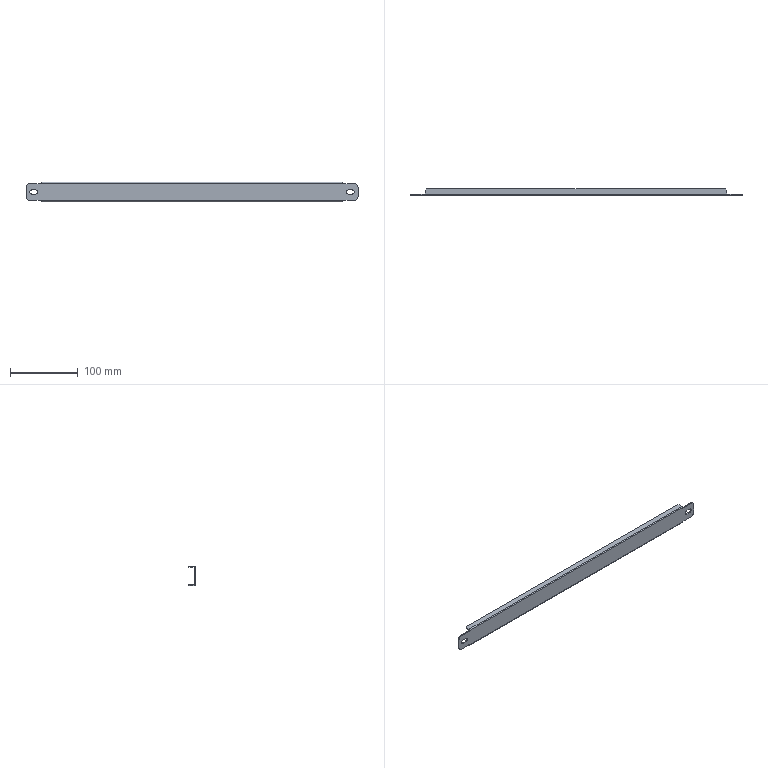Part | SolidWorks | features CornerTrim 2, ICE 2, EdgeFlange 1, FlatPattern 1, SMBaseFlange 1, SheetMetal 1 | 1 solid | 46 faces | box 490 x 9.5 x 29 mm | volume 30933 mm3 | plane 34 | cylinder 12 | commonest cylinder face diameters 6 x4 10 x4 0.2 x2 3.2 x2
STEP:
#1=CARTESIAN_POINT('',(222.5,-1.5,12.));
#2=VERTEX_POINT('',#1);
#3=CARTESIAN_POINT('',(240.,-1.5,12.));
#4=VERTEX_POINT('',#3);
#5=CARTESIAN_POINT('',(-245.,-1.5,12.));
#6=DIRECTION('',(1.,0.,0.));
#7=VECTOR('',#6,1000.);
#8=LINE('',#5,#7);
#9=EDGE_CURVE('',#2,#4,#8,.T.);
#10=ORIENTED_EDGE('',*,*,#9,.T.);
#11=CARTESIAN_POINT('',(240.,0.,12.));
#12=VERTEX_POINT('',#11);
#13=CARTESIAN_POINT('',(240.,-1.5,12.));
#14=DIRECTION('',(0.,1.,0.));
#15=VECTOR('',#14,1000.);
#16=LINE('',#13,#15);
#17=EDGE_CURVE('',#4,#12,#16,.T.);
#18=ORIENTED_EDGE('',*,*,#17,.T.);
#19=CARTESIAN_POINT('',(222.5,0.,12.));
#20=VERTEX_POINT('',#19);
#21=CARTESIAN_POINT('',(-245.,0.,12.));
#22=DIRECTION('',(1.,0.,0.));
#23=VECTOR('',#22,1000.);
#24=LINE('',#21,#23);
#25=EDGE_CURVE('',#20,#12,#24,.T.);
#26=ORIENTED_EDGE('',*,*,#25,.F.);
#27=CARTESIAN_POINT('',(222.5,0.,12.));
#28=DIRECTION('',(0.,-1.,0.));
#29=VECTOR('',#28,1000.);
#30=LINE('',#27,#29);
#31=EDGE_CURVE('',#20,#2,#30,.T.);
#32=ORIENTED_EDGE('',*,*,#31,.T.);
#33=EDGE_LOOP('',(#10,#18,#26,#32));
#34=FACE_OUTER_BOUND('',#33,.T.);
#35=CARTESIAN_POINT('',(-245.,-1.5,12.));
#36=DIRECTION('',(0.,0.,1.));
#37=DIRECTION('',(1.,0.,0.));
#38=AXIS2_PLACEMENT_3D('',#35,#36,#37);
#39=PLANE('',#38);
#40=ADVANCED_FACE('',(#34),#39,.T.);
#41=CARTESIAN_POINT('',(-222.5,-1.5,-12.));
#42=VERTEX_POINT('',#41);
#43=CARTESIAN_POINT('',(-240.,-1.5,-12.));
#44=VERTEX_POINT('',#43);
#45=CARTESIAN_POINT('',(-245.,-1.5,-12.));
#46=DIRECTION('',(-1.,0.,0.));
#47=VECTOR('',#46,1000.);
#48=LINE('',#45,#47);
#49=EDGE_CURVE('',#42,#44,#48,.T.);
#50=ORIENTED_EDGE('',*,*,#49,.T.);
#51=CARTESIAN_POINT('',(-240.,0.,-12.));
#52=VERTEX_POINT('',#51);
#53=CARTESIAN_POINT('',(-240.,-1.5,-12.));
#54=DIRECTION('',(0.,1.,0.));
#55=VECTOR('',#54,1000.);
#56=LINE('',#53,#55);
#57=EDGE_CURVE('',#44,#52,#56,.T.);
#58=ORIENTED_EDGE('',*,*,#57,.T.);
#59=CARTESIAN_POINT('',(-222.5,0.,-12.));
#60=VERTEX_POINT('',#59);
#61=CARTESIAN_POINT('',(-245.,0.,-12.));
#62=DIRECTION('',(-1.,0.,0.));
#63=VECTOR('',#62,1000.);
#64=LINE('',#61,#63);
#65=EDGE_CURVE('',#60,#52,#64,.T.);
#66=ORIENTED_EDGE('',*,*,#65,.F.);
#67=CARTESIAN_POINT('',(-222.5,0.,-12.));
#68=DIRECTION('',(0.,-1.,0.));
#69=VECTOR('',#68,1000.);
#70=LINE('',#67,#69);
#71=EDGE_CURVE('',#60,#42,#70,.T.);
#72=ORIENTED_EDGE('',*,*,#71,.T.);
#73=EDGE_LOOP('',(#50,#58,#66,#72));
#74=FACE_OUTER_BOUND('',#73,.T.);
#75=CARTESIAN_POINT('',(-245.,-1.5,-12.));
#76=DIRECTION('',(0.,0.,-1.));
#77=DIRECTION('',(-1.,0.,0.));
#78=AXIS2_PLACEMENT_3D('',#75,#76,#77);
#79=PLANE('',#78);
#80=ADVANCED_FACE('',(#74),#79,.T.);
#81=CARTESIAN_POINT('',(245.,0.,7.));
#82=VERTEX_POINT('',#81);
#83=CARTESIAN_POINT('',(245.,0.,-7.));
#84=VERTEX_POINT('',#83);
#85=CARTESIAN_POINT('',(245.,0.,-12.));
#86=DIRECTION('',(0.,0.,-1.));
#87=VECTOR('',#86,1000.);
#88=LINE('',#85,#87);
#89=EDGE_CURVE('',#82,#84,#88,.T.);
#90=ORIENTED_EDGE('',*,*,#89,.F.);
#91=CARTESIAN_POINT('',(245.,-1.5,7.));
#92=VERTEX_POINT('',#91);
#93=CARTESIAN_POINT('',(245.,-1.5,7.));
#94=DIRECTION('',(0.,-1.,0.));
#95=VECTOR('',#94,1000.);
#96=LINE('',#93,#95);
#97=EDGE_CURVE('',#82,#92,#96,.T.);
#98=ORIENTED_EDGE('',*,*,#97,.T.);
#99=CARTESIAN_POINT('',(245.,-1.5,-7.));
#100=VERTEX_POINT('',#99);
#101=CARTESIAN_POINT('',(245.,-1.5,-12.));
#102=DIRECTION('',(0.,0.,-1.));
#103=VECTOR('',#102,1000.);
#104=LINE('',#101,#103);
#105=EDGE_CURVE('',#92,#100,#104,.T.);
#106=ORIENTED_EDGE('',*,*,#105,.T.);
#107=CARTESIAN_POINT('',(245.,-1.5,-7.));
#108=DIRECTION('',(0.,1.,0.));
#109=VECTOR('',#108,1000.);
#110=LINE('',#107,#109);
#111=EDGE_CURVE('',#100,#84,#110,.T.);
#112=ORIENTED_EDGE('',*,*,#111,.T.);
#113=EDGE_LOOP('',(#90,#98,#106,#112));
#114=FACE_OUTER_BOUND('',#113,.T.);
#115=CARTESIAN_POINT('',(245.,-1.5,-12.));
#116=DIRECTION('',(1.,0.,0.));
#117=DIRECTION('',(0.,0.,-1.));
#118=AXIS2_PLACEMENT_3D('',#115,#116,#117);
#119=PLANE('',#118);
#120=ADVANCED_FACE('',(#114),#119,.T.);
#121=CARTESIAN_POINT('',(-240.,0.,12.));
#122=VERTEX_POINT('',#121);
#123=CARTESIAN_POINT('',(-222.5,0.,12.));
#124=VERTEX_POINT('',#123);
#125=CARTESIAN_POINT('',(-245.,0.,12.));
#126=DIRECTION('',(1.,0.,0.));
#127=VECTOR('',#126,1000.);
#128=LINE('',#125,#127);
#129=EDGE_CURVE('',#122,#124,#128,.T.);
#130=ORIENTED_EDGE('',*,*,#129,.F.);
#131=CARTESIAN_POINT('',(-240.,-1.5,12.));
#132=VERTEX_POINT('',#131);
#133=CARTESIAN_POINT('',(-240.,-1.5,12.));
#134=DIRECTION('',(0.,-1.,0.));
#135=VECTOR('',#134,1000.);
#136=LINE('',#133,#135);
#137=EDGE_CURVE('',#122,#132,#136,.T.);
#138=ORIENTED_EDGE('',*,*,#137,.T.);
#139=CARTESIAN_POINT('',(-222.5,-1.5,12.));
#140=VERTEX_POINT('',#139);
#141=CARTESIAN_POINT('',(-245.,-1.5,12.));
#142=DIRECTION('',(1.,0.,0.));
#143=VECTOR('',#142,1000.);
#144=LINE('',#141,#143);
#145=EDGE_CURVE('',#132,#140,#144,.T.);
#146=ORIENTED_EDGE('',*,*,#145,.T.);
#147=CARTESIAN_POINT('',(-222.5,0.,12.));
#148=DIRECTION('',(0.,-1.,0.));
#149=VECTOR('',#148,1000.);
#150=LINE('',#147,#149);
#151=EDGE_CURVE('',#124,#140,#150,.T.);
#152=ORIENTED_EDGE('',*,*,#151,.F.);
#153=EDGE_LOOP('',(#130,#138,#146,#152));
#154=FACE_OUTER_BOUND('',#153,.T.);
#155=CARTESIAN_POINT('',(-245.,-1.5,12.));
#156=DIRECTION('',(0.,0.,1.));
#157=DIRECTION('',(1.,0.,0.));
#158=AXIS2_PLACEMENT_3D('',#155,#156,#157);
#159=PLANE('',#158);
#160=ADVANCED_FACE('',(#154),#159,.T.);
#161=CARTESIAN_POINT('',(-245.,-1.5,-7.));
#162=VERTEX_POINT('',#161);
#163=CARTESIAN_POINT('',(-245.,-1.5,7.));
#164=VERTEX_POINT('',#163);
#165=CARTESIAN_POINT('',(-245.,-1.5,-12.));
#166=DIRECTION('',(0.,0.,1.));
#167=VECTOR('',#166,1000.);
#168=LINE('',#165,#167);
#169=EDGE_CURVE('',#162,#164,#168,.T.);
#170=ORIENTED_EDGE('',*,*,#169,.T.);
#171=CARTESIAN_POINT('',(-245.,0.,7.));
#172=VERTEX_POINT('',#171);
#173=CARTESIAN_POINT('',(-245.,-1.5,7.));
#174=DIRECTION('',(0.,1.,0.));
#175=VECTOR('',#174,1000.);
#176=LINE('',#173,#175);
#177=EDGE_CURVE('',#164,#172,#176,.T.);
#178=ORIENTED_EDGE('',*,*,#177,.T.);
#179=CARTESIAN_POINT('',(-245.,0.,-7.));
#180=VERTEX_POINT('',#179);
#181=CARTESIAN_POINT('',(-245.,0.,-12.));
#182=DIRECTION('',(0.,0.,1.));
#183=VECTOR('',#182,1000.);
#184=LINE('',#181,#183);
#185=EDGE_CURVE('',#180,#172,#184,.T.);
#186=ORIENTED_EDGE('',*,*,#185,.F.);
#187=CARTESIAN_POINT('',(-245.,-1.5,-7.));
#188=DIRECTION('',(0.,-1.,0.));
#189=VECTOR('',#188,1000.);
#190=LINE('',#187,#189);
#191=EDGE_CURVE('',#180,#162,#190,.T.);
#192=ORIENTED_EDGE('',*,*,#191,.T.);
#193=EDGE_LOOP('',(#170,#178,#186,#192));
#194=FACE_OUTER_BOUND('',#193,.T.);
#195=CARTESIAN_POINT('',(-245.,-1.5,-12.));
#196=DIRECTION('',(-1.,0.,0.));
#197=DIRECTION('',(0.,0.,1.));
#198=AXIS2_PLACEMENT_3D('',#195,#196,#197);
#199=PLANE('',#198);
#200=ADVANCED_FACE('',(#194),#199,.T.);
#201=CARTESIAN_POINT('',(240.,0.,-12.));
#202=VERTEX_POINT('',#201);
#203=CARTESIAN_POINT('',(222.5,0.,-12.));
#204=VERTEX_POINT('',#203);
#205=CARTESIAN_POINT('',(-245.,0.,-12.));
#206=DIRECTION('',(-1.,0.,0.));
#207=VECTOR('',#206,1000.);
#208=LINE('',#205,#207);
#209=EDGE_CURVE('',#202,#204,#208,.T.);
#210=ORIENTED_EDGE('',*,*,#209,.F.);
#211=CARTESIAN_POINT('',(240.,-1.5,-12.));
#212=VERTEX_POINT('',#211);
#213=CARTESIAN_POINT('',(240.,-1.5,-12.));
#214=DIRECTION('',(0.,-1.,0.));
#215=VECTOR('',#214,1000.);
#216=LINE('',#213,#215);
#217=EDGE_CURVE('',#202,#212,#216,.T.);
#218=ORIENTED_EDGE('',*,*,#217,.T.);
#219=CARTESIAN_POINT('',(222.5,-1.5,-12.));
#220=VERTEX_POINT('',#219);
#221=CARTESIAN_POINT('',(-245.,-1.5,-12.));
#222=DIRECTION('',(-1.,0.,0.));
#223=VECTOR('',#222,1000.);
#224=LINE('',#221,#223);
#225=EDGE_CURVE('',#212,#220,#224,.T.);
#226=ORIENTED_EDGE('',*,*,#225,.T.);
#227=CARTESIAN_POINT('',(222.5,0.,-12.));
#228=DIRECTION('',(0.,-1.,0.));
#229=VECTOR('',#228,1000.);
#230=LINE('',#227,#229);
#231=EDGE_CURVE('',#204,#220,#230,.T.);
#232=ORIENTED_EDGE('',*,*,#231,.F.);
#233=EDGE_LOOP('',(#210,#218,#226,#232));
#234=FACE_OUTER_BOUND('',#233,.T.);
#235=CARTESIAN_POINT('',(-245.,-1.5,-12.));
#236=DIRECTION('',(0.,0.,-1.));
#237=DIRECTION('',(-1.,0.,0.));
#238=AXIS2_PLACEMENT_3D('',#235,#236,#237);
#239=PLANE('',#238);
#240=ADVANCED_FACE('',(#234),#239,.T.);
#241=CARTESIAN_POINT('',(230.5,-1.5,3.));
#242=VERTEX_POINT('',#241);
#243=CARTESIAN_POINT('',(236.5,-1.5,3.));
#244=VERTEX_POINT('',#243);
#245=CARTESIAN_POINT('',(0.,-1.5,3.));
#246=DIRECTION('',(1.,0.,0.));
#247=VECTOR('',#246,1000.);
#248=LINE('',#245,#247);
#249=EDGE_CURVE('',#242,#244,#248,.T.);
#250=ORIENTED_EDGE('',*,*,#249,.T.);
#251=CARTESIAN_POINT('',(236.5,-1.5,-3.));
#252=VERTEX_POINT('',#251);
#253=CARTESIAN_POINT('',(236.5,-1.5,0.));
#254=DIRECTION('',(0.,1.,0.));
#255=DIRECTION('',(0.,0.,1.));
#256=AXIS2_PLACEMENT_3D('',#253,#254,#255);
#257=CIRCLE('',#256,3.);
#258=EDGE_CURVE('',#244,#252,#257,.T.);
#259=ORIENTED_EDGE('',*,*,#258,.T.);
#260=CARTESIAN_POINT('',(230.5,-1.5,-3.));
#261=VERTEX_POINT('',#260);
#262=CARTESIAN_POINT('',(0.,-1.5,-3.));
#263=DIRECTION('',(-1.,0.,0.));
#264=VECTOR('',#263,1000.);
#265=LINE('',#262,#264);
#266=EDGE_CURVE('',#252,#261,#265,.T.);
#267=ORIENTED_EDGE('',*,*,#266,.T.);
#268=CARTESIAN_POINT('',(230.5,-1.5,0.));
#269=DIRECTION('',(0.,1.,0.));
#270=DIRECTION('',(0.,0.,1.));
#271=AXIS2_PLACEMENT_3D('',#268,#269,#270);
#272=CIRCLE('',#271,3.);
#273=EDGE_CURVE('',#261,#242,#272,.T.);
#274=ORIENTED_EDGE('',*,*,#273,.T.);
#275=EDGE_LOOP('',(#250,#259,#267,#274));
#276=FACE_BOUND('',#275,.T.);
#277=CARTESIAN_POINT('',(-236.5,-1.5,3.));
#278=VERTEX_POINT('',#277);
#279=CARTESIAN_POINT('',(-230.5,-1.5,3.));
#280=VERTEX_POINT('',#279);
#281=CARTESIAN_POINT('',(0.,-1.5,3.));
#282=DIRECTION('',(1.,0.,0.));
#283=VECTOR('',#282,1000.);
#284=LINE('',#281,#283);
#285=EDGE_CURVE('',#278,#280,#284,.T.);
#286=ORIENTED_EDGE('',*,*,#285,.T.);
#287=CARTESIAN_POINT('',(-230.5,-1.5,-3.));
#288=VERTEX_POINT('',#287);
#289=CARTESIAN_POINT('',(-230.5,-1.5,0.));
#290=DIRECTION('',(0.,1.,0.));
#291=DIRECTION('',(0.,0.,1.));
#292=AXIS2_PLACEMENT_3D('',#289,#290,#291);
#293=CIRCLE('',#292,3.);
#294=EDGE_CURVE('',#280,#288,#293,.T.);
#295=ORIENTED_EDGE('',*,*,#294,.T.);
#296=CARTESIAN_POINT('',(-236.5,-1.5,-3.));
#297=VERTEX_POINT('',#296);
#298=CARTESIAN_POINT('',(0.,-1.5,-3.));
#299=DIRECTION('',(-1.,0.,0.));
#300=VECTOR('',#299,1000.);
#301=LINE('',#298,#300);
#302=EDGE_CURVE('',#288,#297,#301,.T.);
#303=ORIENTED_EDGE('',*,*,#302,.T.);
#304=CARTESIAN_POINT('',(-236.5,-1.5,0.));
#305=DIRECTION('',(0.,1.,0.));
#306=DIRECTION('',(0.,0.,1.));
#307=AXIS2_PLACEMENT_3D('',#304,#305,#306);
#308=CIRCLE('',#307,3.);
#309=EDGE_CURVE('',#297,#278,#308,.T.);
#310=ORIENTED_EDGE('',*,*,#309,.T.);
#311=EDGE_LOOP('',(#286,#295,#303,#310));
#312=FACE_BOUND('',#311,.T.);
#313=ORIENTED_EDGE('',*,*,#105,.F.);
#314=CARTESIAN_POINT('',(240.,-1.5,7.));
#315=DIRECTION('',(0.,-1.,0.));
#316=DIRECTION('',(0.,0.,1.));
#317=AXIS2_PLACEMENT_3D('',#314,#315,#316);
#318=CIRCLE('',#317,5.);
#319=EDGE_CURVE('',#92,#4,#318,.T.);
#320=ORIENTED_EDGE('',*,*,#319,.T.);
#321=ORIENTED_EDGE('',*,*,#9,.F.);
#322=CARTESIAN_POINT('',(222.5,-1.5,12.9));
#323=VERTEX_POINT('',#322);
#324=CARTESIAN_POINT('',(222.5,-1.5,12.9));
#325=DIRECTION('',(0.,0.,-1.));
#326=VECTOR('',#325,1000.);
#327=LINE('',#324,#326);
#328=EDGE_CURVE('',#323,#2,#327,.T.);
#329=ORIENTED_EDGE('',*,*,#328,.F.);
#330=CARTESIAN_POINT('',(-222.5,-1.5,12.9));
#331=VERTEX_POINT('',#330);
#332=CARTESIAN_POINT('',(222.5,-1.5,12.9));
#333=DIRECTION('',(-1.,0.,0.));
#334=VECTOR('',#333,1000.);
#335=LINE('',#332,#334);
#336=EDGE_CURVE('',#323,#331,#335,.T.);
#337=ORIENTED_EDGE('',*,*,#336,.T.);
#338=CARTESIAN_POINT('',(-222.5,-1.5,12.9));
#339=DIRECTION('',(0.,0.,-1.));
#340=VECTOR('',#339,1000.);
#341=LINE('',#338,#340);
#342=EDGE_CURVE('',#331,#140,#341,.T.);
#343=ORIENTED_EDGE('',*,*,#342,.T.);
#344=ORIENTED_EDGE('',*,*,#145,.F.);
#345=CARTESIAN_POINT('',(-240.,-1.5,7.));
#346=DIRECTION('',(0.,-1.,0.));
#347=DIRECTION('',(0.,0.,1.));
#348=AXIS2_PLACEMENT_3D('',#345,#346,#347);
#349=CIRCLE('',#348,5.);
#350=EDGE_CURVE('',#132,#164,#349,.T.);
#351=ORIENTED_EDGE('',*,*,#350,.T.);
#352=ORIENTED_EDGE('',*,*,#169,.F.);
#353=CARTESIAN_POINT('',(-240.,-1.5,-7.));
#354=DIRECTION('',(0.,-1.,0.));
#355=DIRECTION('',(0.,0.,1.));
#356=AXIS2_PLACEMENT_3D('',#353,#354,#355);
#357=CIRCLE('',#356,5.);
#358=EDGE_CURVE('',#162,#44,#357,.T.);
#359=ORIENTED_EDGE('',*,*,#358,.T.);
#360=ORIENTED_EDGE('',*,*,#49,.F.);
#361=CARTESIAN_POINT('',(-222.5,-1.5,-12.9));
#362=VERTEX_POINT('',#361);
#363=CARTESIAN_POINT('',(-222.5,-1.5,-12.9));
#364=DIRECTION('',(0.,0.,1.));
#365=VECTOR('',#364,1000.);
#366=LINE('',#363,#365);
#367=EDGE_CURVE('',#362,#42,#366,.T.);
#368=ORIENTED_EDGE('',*,*,#367,.F.);
#369=CARTESIAN_POINT('',(222.5,-1.5,-12.9));
#370=VERTEX_POINT('',#369);
#371=CARTESIAN_POINT('',(-222.5,-1.5,-12.9));
#372=DIRECTION('',(1.,0.,0.));
#373=VECTOR('',#372,1000.);
#374=LINE('',#371,#373);
#375=EDGE_CURVE('',#362,#370,#374,.T.);
#376=ORIENTED_EDGE('',*,*,#375,.T.);
#377=CARTESIAN_POINT('',(222.5,-1.5,-12.9));
#378=DIRECTION('',(0.,0.,1.));
#379=VECTOR('',#378,1000.);
#380=LINE('',#377,#379);
#381=EDGE_CURVE('',#370,#220,#380,.T.);
#382=ORIENTED_EDGE('',*,*,#381,.T.);
#383=ORIENTED_EDGE('',*,*,#225,.F.);
#384=CARTESIAN_POINT('',(240.,-1.5,-7.));
#385=DIRECTION('',(0.,-1.,0.));
#386=DIRECTION('',(0.,0.,1.));
#387=AXIS2_PLACEMENT_3D('',#384,#385,#386);
#388=CIRCLE('',#387,5.);
#389=EDGE_CURVE('',#212,#100,#388,.T.);
#390=ORIENTED_EDGE('',*,*,#389,.T.);
#391=EDGE_LOOP('',(#313,#320,#321,#329,#337,#343,#344,#351,#352,#359,#360,#368,#376,#382,#383,#390));
#392=FACE_OUTER_BOUND('',#391,.T.);
#393=CARTESIAN_POINT('',(0.,-1.5,0.));
#394=DIRECTION('',(0.,1.,0.));
#395=DIRECTION('',(0.,0.,1.));
#396=AXIS2_PLACEMENT_3D('',#393,#394,#395);
#397=PLANE('',#396);
#398=ADVANCED_FACE('',(#276,#312,#392),#397,.F.);
#399=CARTESIAN_POINT('',(236.5,0.,3.));
#400=VERTEX_POINT('',#399);
#401=CARTESIAN_POINT('',(236.5,0.,-3.));
#402=VERTEX_POINT('',#401);
#403=CARTESIAN_POINT('',(236.5,0.,0.));
#404=DIRECTION('',(0.,1.,0.));
#405=DIRECTION('',(0.,0.,1.));
#406=AXIS2_PLACEMENT_3D('',#403,#404,#405);
#407=CIRCLE('',#406,3.);
#408=EDGE_CURVE('',#400,#402,#407,.T.);
#409=ORIENTED_EDGE('',*,*,#408,.F.);
#410=CARTESIAN_POINT('',(230.5,0.,3.));
#411=VERTEX_POINT('',#410);
#412=CARTESIAN_POINT('',(236.5,0.,3.));
#413=DIRECTION('',(1.,0.,0.));
#414=VECTOR('',#413,1000.);
#415=LINE('',#412,#414);
#416=EDGE_CURVE('',#411,#400,#415,.T.);
#417=ORIENTED_EDGE('',*,*,#416,.F.);
#418=CARTESIAN_POINT('',(230.5,0.,-3.));
#419=VERTEX_POINT('',#418);
#420=CARTESIAN_POINT('',(230.5,0.,0.));
#421=DIRECTION('',(0.,1.,0.));
#422=DIRECTION('',(0.,0.,1.));
#423=AXIS2_PLACEMENT_3D('',#420,#421,#422);
#424=CIRCLE('',#423,3.);
#425=EDGE_CURVE('',#419,#411,#424,.T.);
#426=ORIENTED_EDGE('',*,*,#425,.F.);
#427=CARTESIAN_POINT('',(236.5,0.,-3.));
#428=DIRECTION('',(-1.,0.,0.));
#429=VECTOR('',#428,1000.);
#430=LINE('',#427,#429);
#431=EDGE_CURVE('',#402,#419,#430,.T.);
#432=ORIENTED_EDGE('',*,*,#431,.F.);
#433=EDGE_LOOP('',(#409,#417,#426,#432));
#434=FACE_BOUND('',#433,.T.);
#435=CARTESIAN_POINT('',(-230.5,0.,3.));
#436=VERTEX_POINT('',#435);
#437=CARTESIAN_POINT('',(-230.5,0.,-3.));
#438=VERTEX_POINT('',#437);
#439=CARTESIAN_POINT('',(-230.5,0.,0.));
#440=DIRECTION('',(0.,1.,0.));
#441=DIRECTION('',(0.,0.,1.));
#442=AXIS2_PLACEMENT_3D('',#439,#440,#441);
#443=CIRCLE('',#442,3.);
#444=EDGE_CURVE('',#436,#438,#443,.T.);
#445=ORIENTED_EDGE('',*,*,#444,.F.);
#446=CARTESIAN_POINT('',(-236.5,0.,3.));
#447=VERTEX_POINT('',#446);
#448=CARTESIAN_POINT('',(-230.5,0.,3.));
#449=DIRECTION('',(1.,0.,0.));
#450=VECTOR('',#449,1000.);
#451=LINE('',#448,#450);
#452=EDGE_CURVE('',#447,#436,#451,.T.);
#453=ORIENTED_EDGE('',*,*,#452,.F.);
#454=CARTESIAN_POINT('',(-236.5,0.,-3.));
#455=VERTEX_POINT('',#454);
#456=CARTESIAN_POINT('',(-236.5,0.,0.));
#457=DIRECTION('',(0.,1.,0.));
#458=DIRECTION('',(0.,0.,1.));
#459=AXIS2_PLACEMENT_3D('',#456,#457,#458);
#460=CIRCLE('',#459,3.);
#461=EDGE_CURVE('',#455,#447,#460,.T.);
#462=ORIENTED_EDGE('',*,*,#461,.F.);
#463=CARTESIAN_POINT('',(-230.5,0.,-3.));
#464=DIRECTION('',(-1.,0.,0.));
#465=VECTOR('',#464,1000.);
#466=LINE('',#463,#465);
#467=EDGE_CURVE('',#438,#455,#466,.T.);
#468=ORIENTED_EDGE('',*,*,#467,.F.);
#469=EDGE_LOOP('',(#445,#453,#462,#468));
#470=FACE_BOUND('',#469,.T.);
#471=ORIENTED_EDGE('',*,*,#25,.T.);
#472=CARTESIAN_POINT('',(240.,0.,7.));
#473=DIRECTION('',(0.,1.,0.));
#474=DIRECTION('',(0.,0.,1.));
#475=AXIS2_PLACEMENT_3D('',#472,#473,#474);
#476=CIRCLE('',#475,5.);
#477=EDGE_CURVE('',#12,#82,#476,.T.);
#478=ORIENTED_EDGE('',*,*,#477,.T.);
#479=ORIENTED_EDGE('',*,*,#89,.T.);
#480=CARTESIAN_POINT('',(240.,0.,-7.));
#481=DIRECTION('',(0.,1.,0.));
#482=DIRECTION('',(0.,0.,1.));
#483=AXIS2_PLACEMENT_3D('',#480,#481,#482);
#484=CIRCLE('',#483,5.);
#485=EDGE_CURVE('',#84,#202,#484,.T.);
#486=ORIENTED_EDGE('',*,*,#485,.T.);
#487=ORIENTED_EDGE('',*,*,#209,.T.);
#488=CARTESIAN_POINT('',(222.5,0.,-12.9));
#489=VERTEX_POINT('',#488);
#490=CARTESIAN_POINT('',(222.5,0.,-12.9));
#491=DIRECTION('',(0.,0.,1.));
#492=VECTOR('',#491,1000.);
#493=LINE('',#490,#492);
#494=EDGE_CURVE('',#489,#204,#493,.T.);
#495=ORIENTED_EDGE('',*,*,#494,.F.);
#496=CARTESIAN_POINT('',(-222.5,0.,-12.9));
#497=VERTEX_POINT('',#496);
#498=CARTESIAN_POINT('',(-222.5,0.,-12.9));
#499=DIRECTION('',(1.,0.,0.));
#500=VECTOR('',#499,1000.);
#501=LINE('',#498,#500);
#502=EDGE_CURVE('',#497,#489,#501,.T.);
#503=ORIENTED_EDGE('',*,*,#502,.F.);
#504=CARTESIAN_POINT('',(-222.5,0.,-12.9));
#505=DIRECTION('',(0.,0.,1.));
#506=VECTOR('',#505,1000.);
#507=LINE('',#504,#506);
#508=EDGE_CURVE('',#497,#60,#507,.T.);
#509=ORIENTED_EDGE('',*,*,#508,.T.);
#510=ORIENTED_EDGE('',*,*,#65,.T.);
#511=CARTESIAN_POINT('',(-240.,0.,-7.));
#512=DIRECTION('',(0.,1.,0.));
#513=DIRECTION('',(0.,0.,1.));
#514=AXIS2_PLACEMENT_3D('',#511,#512,#513);
#515=CIRCLE('',#514,5.);
#516=EDGE_CURVE('',#52,#180,#515,.T.);
#517=ORIENTED_EDGE('',*,*,#516,.T.);
#518=ORIENTED_EDGE('',*,*,#185,.T.);
#519=CARTESIAN_POINT('',(-240.,0.,7.));
#520=DIRECTION('',(0.,1.,0.));
#521=DIRECTION('',(0.,0.,1.));
#522=AXIS2_PLACEMENT_3D('',#519,#520,#521);
#523=CIRCLE('',#522,5.);
#524=EDGE_CURVE('',#172,#122,#523,.T.);
#525=ORIENTED_EDGE('',*,*,#524,.T.);
#526=ORIENTED_EDGE('',*,*,#129,.T.);
#527=CARTESIAN_POINT('',(-222.5,0.,12.9));
#528=VERTEX_POINT('',#527);
#529=CARTESIAN_POINT('',(-222.5,0.,12.9));
#530=DIRECTION('',(0.,0.,-1.));
#531=VECTOR('',#530,1000.);
#532=LINE('',#529,#531);
#533=EDGE_CURVE('',#528,#124,#532,.T.);
#534=ORIENTED_EDGE('',*,*,#533,.F.);
#535=CARTESIAN_POINT('',(222.5,0.,12.9));
#536=VERTEX_POINT('',#535);
#537=CARTESIAN_POINT('',(222.5,0.,12.9));
#538=DIRECTION('',(-1.,0.,0.));
#539=VECTOR('',#538,1000.);
#540=LINE('',#537,#539);
#541=EDGE_CURVE('',#536,#528,#540,.T.);
#542=ORIENTED_EDGE('',*,*,#541,.F.);
#543=CARTESIAN_POINT('',(222.5,0.,12.9));
#544=DIRECTION('',(0.,0.,-1.));
#545=VECTOR('',#544,1000.);
#546=LINE('',#543,#545);
#547=EDGE_CURVE('',#536,#20,#546,.T.);
#548=ORIENTED_EDGE('',*,*,#547,.T.);
#549=EDGE_LOOP('',(#471,#478,#479,#486,#487,#495,#503,#509,#510,#517,#518,#525,#526,#534,#542,#548));
#550=FACE_OUTER_BOUND('',#549,.T.);
#551=CARTESIAN_POINT('',(0.,0.,0.));
#552=DIRECTION('',(0.,1.,0.));
#553=DIRECTION('',(0.,0.,1.));
#554=AXIS2_PLACEMENT_3D('',#551,#552,#553);
#555=PLANE('',#554);
#556=ADVANCED_FACE('',(#434,#470,#550),#555,.T.);
#557=ORIENTED_EDGE('',*,*,#508,.F.);
#558=CARTESIAN_POINT('',(-222.5,0.,-12.9));
#559=DIRECTION('',(0.,-1.,0.));
#560=VECTOR('',#559,1000.);
#561=LINE('',#558,#560);
#562=EDGE_CURVE('',#497,#362,#561,.T.);
#563=ORIENTED_EDGE('',*,*,#562,.T.);
#564=ORIENTED_EDGE('',*,*,#367,.T.);
#565=ORIENTED_EDGE('',*,*,#71,.F.);
#566=EDGE_LOOP('',(#557,#563,#564,#565));
#567=FACE_OUTER_BOUND('',#566,.T.);
#568=CARTESIAN_POINT('',(-222.5,0.,-12.9));
#569=DIRECTION('',(-1.,0.,0.));
#570=DIRECTION('',(0.,-1.,0.));
#571=AXIS2_PLACEMENT_3D('',#568,#569,#570);
#572=PLANE('',#571);
#573=ADVANCED_FACE('',(#567),#572,.T.);
#574=ORIENTED_EDGE('',*,*,#381,.F.);
#575=CARTESIAN_POINT('',(222.5,0.,-12.9));
#576=DIRECTION('',(0.,-1.,0.));
#577=VECTOR('',#576,1000.);
#578=LINE('',#575,#577);
#579=EDGE_CURVE('',#489,#370,#578,.T.);
#580=ORIENTED_EDGE('',*,*,#579,.F.);
#581=ORIENTED_EDGE('',*,*,#494,.T.);
#582=ORIENTED_EDGE('',*,*,#231,.T.);
#583=EDGE_LOOP('',(#574,#580,#581,#582));
#584=FACE_OUTER_BOUND('',#583,.T.);
#585=CARTESIAN_POINT('',(222.5,0.,-12.9));
#586=DIRECTION('',(-1.,0.,0.));
#587=DIRECTION('',(0.,-1.,0.));
#588=AXIS2_PLACEMENT_3D('',#585,#586,#587);
#589=PLANE('',#588);
#590=ADVANCED_FACE('',(#584),#589,.F.);
#591=ORIENTED_EDGE('',*,*,#547,.F.);
#592=CARTESIAN_POINT('',(222.5,0.,12.9));
#593=DIRECTION('',(0.,-1.,0.));
#594=VECTOR('',#593,1000.);
#595=LINE('',#592,#594);
#596=EDGE_CURVE('',#536,#323,#595,.T.);
#597=ORIENTED_EDGE('',*,*,#596,.T.);
#598=ORIENTED_EDGE('',*,*,#328,.T.);
#599=ORIENTED_EDGE('',*,*,#31,.F.);
#600=EDGE_LOOP('',(#591,#597,#598,#599));
#601=FACE_OUTER_BOUND('',#600,.T.);
#602=CARTESIAN_POINT('',(222.5,0.,12.9));
#603=DIRECTION('',(1.,0.,0.));
#604=DIRECTION('',(0.,-1.,0.));
#605=AXIS2_PLACEMENT_3D('',#602,#603,#604);
#606=PLANE('',#605);
#607=ADVANCED_FACE('',(#601),#606,.T.);
#608=ORIENTED_EDGE('',*,*,#342,.F.);
#609=CARTESIAN_POINT('',(-222.5,0.,12.9));
#610=DIRECTION('',(0.,-1.,0.));
#611=VECTOR('',#610,1000.);
#612=LINE('',#609,#611);
#613=EDGE_CURVE('',#528,#331,#612,.T.);
#614=ORIENTED_EDGE('',*,*,#613,.F.);
#615=ORIENTED_EDGE('',*,*,#533,.T.);
#616=ORIENTED_EDGE('',*,*,#151,.T.);
#617=EDGE_LOOP('',(#608,#614,#615,#616));
#618=FACE_OUTER_BOUND('',#617,.T.);
#619=CARTESIAN_POINT('',(-222.5,0.,12.9));
#620=DIRECTION('',(1.,0.,0.));
#621=DIRECTION('',(0.,-1.,0.));
#622=AXIS2_PLACEMENT_3D('',#619,#620,#621);
#623=PLANE('',#622);
#624=ADVANCED_FACE('',(#618),#623,.F.);
#625=CARTESIAN_POINT('',(222.5,0.1,-13.));
#626=VERTEX_POINT('',#625);
#627=CARTESIAN_POINT('',(222.5,0.1,-14.5));
#628=VERTEX_POINT('',#627);
#629=CARTESIAN_POINT('',(222.5,0.1,-14.5));
#630=DIRECTION('',(0.,0.,-1.));
#631=VECTOR('',#630,1000.);
#632=LINE('',#629,#631);
#633=EDGE_CURVE('',#626,#628,#632,.T.);
#634=ORIENTED_EDGE('',*,*,#633,.F.);
#635=CARTESIAN_POINT('',(222.5,0.1,-12.9));
#636=DIRECTION('',(1.,0.,0.));
#637=DIRECTION('',(0.,-1.,0.));
#638=AXIS2_PLACEMENT_3D('',#635,#636,#637);
#639=CIRCLE('',#638,0.1);
#640=EDGE_CURVE('',#489,#626,#639,.T.);
#641=ORIENTED_EDGE('',*,*,#640,.F.);
#642=ORIENTED_EDGE('',*,*,#579,.T.);
#643=CARTESIAN_POINT('',(222.5,0.1,-12.9));
#644=DIRECTION('',(1.,0.,0.));
#645=DIRECTION('',(0.,-1.,0.));
#646=AXIS2_PLACEMENT_3D('',#643,#644,#645);
#647=CIRCLE('',#646,1.6);
#648=EDGE_CURVE('',#370,#628,#647,.T.);
#649=ORIENTED_EDGE('',*,*,#648,.T.);
#650=EDGE_LOOP('',(#634,#641,#642,#649));
#651=FACE_OUTER_BOUND('',#650,.T.);
#652=CARTESIAN_POINT('',(222.5,0.1,-12.9));
#653=DIRECTION('',(1.,0.,0.));
#654=DIRECTION('',(0.,1.,0.));
#655=AXIS2_PLACEMENT_3D('',#652,#653,#654);
#656=PLANE('',#655);
#657=ADVANCED_FACE('',(#651),#656,.T.);
#658=CARTESIAN_POINT('',(-222.5,0.1,-13.));
#659=VERTEX_POINT('',#658);
#660=CARTESIAN_POINT('',(-222.5,0.1,-12.9));
#661=DIRECTION('',(-1.,0.,0.));
#662=DIRECTION('',(0.,-1.,0.));
#663=AXIS2_PLACEMENT_3D('',#660,#661,#662);
#664=CIRCLE('',#663,0.1);
#665=EDGE_CURVE('',#659,#497,#664,.T.);
#666=ORIENTED_EDGE('',*,*,#665,.F.);
#667=CARTESIAN_POINT('',(-222.5,0.1,-14.5));
#668=VERTEX_POINT('',#667);
#669=CARTESIAN_POINT('',(-222.5,0.1,-13.));
#670=DIRECTION('',(0.,0.,-1.));
#671=VECTOR('',#670,1000.);
#672=LINE('',#669,#671);
#673=EDGE_CURVE('',#659,#668,#672,.T.);
#674=ORIENTED_EDGE('',*,*,#673,.T.);
#675=CARTESIAN_POINT('',(-222.5,0.1,-12.9));
#676=DIRECTION('',(-1.,0.,0.));
#677=DIRECTION('',(0.,-1.,0.));
#678=AXIS2_PLACEMENT_3D('',#675,#676,#677);
#679=CIRCLE('',#678,1.6);
#680=EDGE_CURVE('',#668,#362,#679,.T.);
#681=ORIENTED_EDGE('',*,*,#680,.T.);
#682=ORIENTED_EDGE('',*,*,#562,.F.);
#683=EDGE_LOOP('',(#666,#674,#681,#682));
#684=FACE_OUTER_BOUND('',#683,.T.);
#685=CARTESIAN_POINT('',(-222.5,0.1,-12.9));
#686=DIRECTION('',(1.,0.,0.));
#687=DIRECTION('',(0.,1.,0.));
#688=AXIS2_PLACEMENT_3D('',#685,#686,#687);
#689=PLANE('',#688);
#690=ADVANCED_FACE('',(#684),#689,.F.);
#691=ORIENTED_EDGE('',*,*,#375,.F.);
#692=ORIENTED_EDGE('',*,*,#680,.F.);
#693=CARTESIAN_POINT('',(222.5,0.1,-14.5));
#694=DIRECTION('',(1.,0.,0.));
#695=VECTOR('',#694,1000.);
#696=LINE('',#693,#695);
#697=EDGE_CURVE('',#668,#628,#696,.T.);
#698=ORIENTED_EDGE('',*,*,#697,.T.);
#699=ORIENTED_EDGE('',*,*,#648,.F.);
#700=EDGE_LOOP('',(#691,#692,#698,#699));
#701=FACE_OUTER_BOUND('',#700,.T.);
#702=CARTESIAN_POINT('',(-222.5,0.1,-12.9));
#703=DIRECTION('',(-1.,0.,0.));
#704=DIRECTION('',(0.,0.,-1.));
#705=AXIS2_PLACEMENT_3D('',#702,#703,#704);
#706=CYLINDRICAL_SURFACE('',#705,1.6);
#707=ADVANCED_FACE('',(#701),#706,.T.);
#708=ORIENTED_EDGE('',*,*,#502,.T.);
#709=ORIENTED_EDGE('',*,*,#640,.T.);
#710=CARTESIAN_POINT('',(222.5,0.1,-13.));
#711=DIRECTION('',(-1.,0.,0.));
#712=VECTOR('',#711,1000.);
#713=LINE('',#710,#712);
#714=EDGE_CURVE('',#626,#659,#713,.T.);
#715=ORIENTED_EDGE('',*,*,#714,.T.);
#716=ORIENTED_EDGE('',*,*,#665,.T.);
#717=EDGE_LOOP('',(#708,#709,#715,#716));
#718=FACE_OUTER_BOUND('',#717,.T.);
#719=CARTESIAN_POINT('',(-222.5,0.1,-12.9));
#720=DIRECTION('',(-1.,0.,0.));
#721=DIRECTION('',(0.,0.,-1.));
#722=AXIS2_PLACEMENT_3D('',#719,#720,#721);
#723=CYLINDRICAL_SURFACE('',#722,0.1);
#724=ADVANCED_FACE('',(#718),#723,.F.);
#725=CARTESIAN_POINT('',(222.5,6.,-14.5));
#726=VERTEX_POINT('',#725);
#727=CARTESIAN_POINT('',(222.5,0.,-14.5));
#728=DIRECTION('',(0.,-1.,0.));
#729=VECTOR('',#728,1000.);
#730=LINE('',#727,#729);
#731=EDGE_CURVE('',#726,#628,#730,.T.);
#732=ORIENTED_EDGE('',*,*,#731,.F.);
#733=CARTESIAN_POINT('',(222.5,6.,-13.));
#734=VERTEX_POINT('',#733);
#735=CARTESIAN_POINT('',(222.5,6.,-14.5));
#736=DIRECTION('',(0.,0.,1.));
#737=VECTOR('',#736,1000.);
#738=LINE('',#735,#737);
#739=EDGE_CURVE('',#726,#734,#738,.T.);
#740=ORIENTED_EDGE('',*,*,#739,.T.);
#741=CARTESIAN_POINT('',(222.5,0.,-13.));
#742=DIRECTION('',(0.,-1.,0.));
#743=VECTOR('',#742,1000.);
#744=LINE('',#741,#743);
#745=EDGE_CURVE('',#734,#626,#744,.T.);
#746=ORIENTED_EDGE('',*,*,#745,.T.);
#747=ORIENTED_EDGE('',*,*,#633,.T.);
#748=EDGE_LOOP('',(#732,#740,#746,#747));
#749=FACE_OUTER_BOUND('',#748,.T.);
#750=CARTESIAN_POINT('',(222.5,0.,-14.5));
#751=DIRECTION('',(-1.,0.,0.));
#752=DIRECTION('',(0.,0.,1.));
#753=AXIS2_PLACEMENT_3D('',#750,#751,#752);
#754=PLANE('',#753);
#755=ADVANCED_FACE('',(#749),#754,.F.);
#756=CARTESIAN_POINT('',(-222.5,6.,-13.));
#757=VERTEX_POINT('',#756);
#758=CARTESIAN_POINT('',(-222.5,8.,-13.));
#759=DIRECTION('',(0.,1.,0.));
#760=VECTOR('',#759,1000.);
#761=LINE('',#758,#760);
#762=EDGE_CURVE('',#659,#757,#761,.T.);
#763=ORIENTED_EDGE('',*,*,#762,.T.);
#764=CARTESIAN_POINT('',(-222.5,6.,-14.5));
#765=VERTEX_POINT('',#764);
#766=CARTESIAN_POINT('',(-222.5,6.,-14.5));
#767=DIRECTION('',(0.,0.,-1.));
#768=VECTOR('',#767,1000.);
#769=LINE('',#766,#768);
#770=EDGE_CURVE('',#757,#765,#769,.T.);
#771=ORIENTED_EDGE('',*,*,#770,.T.);
#772=CARTESIAN_POINT('',(-222.5,0.,-14.5));
#773=DIRECTION('',(0.,1.,0.));
#774=VECTOR('',#773,1000.);
#775=LINE('',#772,#774);
#776=EDGE_CURVE('',#668,#765,#775,.T.);
#777=ORIENTED_EDGE('',*,*,#776,.F.);
#778=ORIENTED_EDGE('',*,*,#673,.F.);
#779=EDGE_LOOP('',(#763,#771,#777,#778));
#780=FACE_OUTER_BOUND('',#779,.T.);
#781=CARTESIAN_POINT('',(-222.5,8.,-14.5));
#782=DIRECTION('',(1.,0.,0.));
#783=DIRECTION('',(0.,0.,-1.));
#784=AXIS2_PLACEMENT_3D('',#781,#782,#783);
#785=PLANE('',#784);
#786=ADVANCED_FACE('',(#780),#785,.F.);
#787=CARTESIAN_POINT('',(-220.5,8.,-14.5));
#788=VERTEX_POINT('',#787);
#789=CARTESIAN_POINT('',(220.5,8.,-14.5));
#790=VERTEX_POINT('',#789);
#791=CARTESIAN_POINT('',(0.,8.,-14.5));
#792=DIRECTION('',(1.,0.,0.));
#793=VECTOR('',#792,1000.);
#794=LINE('',#791,#793);
#795=EDGE_CURVE('',#788,#790,#794,.T.);
#796=ORIENTED_EDGE('',*,*,#795,.T.);
#797=CARTESIAN_POINT('',(222.5,6.,-14.5));
#798=DIRECTION('',(0.7071,-0.7071,0.));
#799=VECTOR('',#798,1000.);
#800=LINE('',#797,#799);
#801=EDGE_CURVE('',#790,#726,#800,.T.);
#802=ORIENTED_EDGE('',*,*,#801,.T.);
#803=ORIENTED_EDGE('',*,*,#731,.T.);
#804=ORIENTED_EDGE('',*,*,#697,.F.);
#805=ORIENTED_EDGE('',*,*,#776,.T.);
#806=CARTESIAN_POINT('',(-220.5,8.,-14.5));
#807=DIRECTION('',(0.7071,0.7071,0.));
#808=VECTOR('',#807,1000.);
#809=LINE('',#806,#808);
#810=EDGE_CURVE('',#765,#788,#809,.T.);
#811=ORIENTED_EDGE('',*,*,#810,.T.);
#812=EDGE_LOOP('',(#796,#802,#803,#804,#805,#811));
#813=FACE_OUTER_BOUND('',#812,.T.);
#814=CARTESIAN_POINT('',(0.,0.,-14.5));
#815=DIRECTION('',(0.,0.,1.));
#816=DIRECTION('',(0.,-1.,0.));
#817=AXIS2_PLACEMENT_3D('',#814,#815,#816);
#818=PLANE('',#817);
#819=ADVANCED_FACE('',(#813),#818,.F.);
#820=ORIENTED_EDGE('',*,*,#745,.F.);
#821=CARTESIAN_POINT('',(220.5,8.,-13.));
#822=VERTEX_POINT('',#821);
#823=CARTESIAN_POINT('',(114.25,114.25,-13.));
#824=DIRECTION('',(-0.7071,0.7071,0.));
#825=VECTOR('',#824,1000.);
#826=LINE('',#823,#825);
#827=EDGE_CURVE('',#734,#822,#826,.T.);
#828=ORIENTED_EDGE('',*,*,#827,.T.);
#829=CARTESIAN_POINT('',(-220.5,8.,-13.));
#830=VERTEX_POINT('',#829);
#831=CARTESIAN_POINT('',(222.5,8.,-13.));
#832=DIRECTION('',(1.,0.,0.));
#833=VECTOR('',#832,1000.);
#834=LINE('',#831,#833);
#835=EDGE_CURVE('',#830,#822,#834,.T.);
#836=ORIENTED_EDGE('',*,*,#835,.F.);
#837=CARTESIAN_POINT('',(-114.25,114.25,-13.));
#838=DIRECTION('',(-0.7071,-0.7071,0.));
#839=VECTOR('',#838,1000.);
#840=LINE('',#837,#839);
#841=EDGE_CURVE('',#830,#757,#840,.T.);
#842=ORIENTED_EDGE('',*,*,#841,.T.);
#843=ORIENTED_EDGE('',*,*,#762,.F.);
#844=ORIENTED_EDGE('',*,*,#714,.F.);
#845=EDGE_LOOP('',(#820,#828,#836,#842,#843,#844));
#846=FACE_OUTER_BOUND('',#845,.T.);
#847=CARTESIAN_POINT('',(0.,0.,-13.));
#848=DIRECTION('',(0.,0.,1.));
#849=DIRECTION('',(0.,-1.,0.));
#850=AXIS2_PLACEMENT_3D('',#847,#848,#849);
#851=PLANE('',#850);
#852=ADVANCED_FACE('',(#846),#851,.T.);
#853=ORIENTED_EDGE('',*,*,#835,.T.);
#854=CARTESIAN_POINT('',(220.5,8.,-14.5));
#855=DIRECTION('',(0.,0.,-1.));
#856=VECTOR('',#855,1000.);
#857=LINE('',#854,#856);
#858=EDGE_CURVE('',#822,#790,#857,.T.);
#859=ORIENTED_EDGE('',*,*,#858,.T.);
#860=ORIENTED_EDGE('',*,*,#795,.F.);
#861=CARTESIAN_POINT('',(-220.5,8.,-14.5));
#862=DIRECTION('',(0.,0.,1.));
#863=VECTOR('',#862,1000.);
#864=LINE('',#861,#863);
#865=EDGE_CURVE('',#788,#830,#864,.T.);
#866=ORIENTED_EDGE('',*,*,#865,.T.);
#867=EDGE_LOOP('',(#853,#859,#860,#866));
#868=FACE_OUTER_BOUND('',#867,.T.);
#869=CARTESIAN_POINT('',(222.5,8.,-14.5));
#870=DIRECTION('',(0.,-1.,0.));
#871=DIRECTION('',(0.,0.,-1.));
#872=AXIS2_PLACEMENT_3D('',#869,#870,#871);
#873=PLANE('',#872);
#874=ADVANCED_FACE('',(#868),#873,.F.);
#875=CARTESIAN_POINT('',(-222.5,0.1,13.));
#876=VERTEX_POINT('',#875);
#877=CARTESIAN_POINT('',(-222.5,0.1,14.5));
#878=VERTEX_POINT('',#877);
#879=CARTESIAN_POINT('',(-222.5,0.1,14.5));
#880=DIRECTION('',(0.,0.,1.));
#881=VECTOR('',#880,1000.);
#882=LINE('',#879,#881);
#883=EDGE_CURVE('',#876,#878,#882,.T.);
#884=ORIENTED_EDGE('',*,*,#883,.F.);
#885=CARTESIAN_POINT('',(-222.5,0.1,12.9));
#886=DIRECTION('',(-1.,0.,0.));
#887=DIRECTION('',(0.,0.,-1.));
#888=AXIS2_PLACEMENT_3D('',#885,#886,#887);
#889=CIRCLE('',#888,0.1);
#890=EDGE_CURVE('',#528,#876,#889,.T.);
#891=ORIENTED_EDGE('',*,*,#890,.F.);
#892=ORIENTED_EDGE('',*,*,#613,.T.);
#893=CARTESIAN_POINT('',(-222.5,0.1,12.9));
#894=DIRECTION('',(-1.,0.,0.));
#895=DIRECTION('',(0.,0.,-1.));
#896=AXIS2_PLACEMENT_3D('',#893,#894,#895);
#897=CIRCLE('',#896,1.6);
#898=EDGE_CURVE('',#331,#878,#897,.T.);
#899=ORIENTED_EDGE('',*,*,#898,.T.);
#900=EDGE_LOOP('',(#884,#891,#892,#899));
#901=FACE_OUTER_BOUND('',#900,.T.);
#902=CARTESIAN_POINT('',(-222.5,0.1,12.9));
#903=DIRECTION('',(-1.,0.,0.));
#904=DIRECTION('',(0.,0.,1.));
#905=AXIS2_PLACEMENT_3D('',#902,#903,#904);
#906=PLANE('',#905);
#907=ADVANCED_FACE('',(#901),#906,.T.);
#908=CARTESIAN_POINT('',(222.5,0.1,13.));
#909=VERTEX_POINT('',#908);
#910=CARTESIAN_POINT('',(222.5,0.1,12.9));
#911=DIRECTION('',(1.,0.,0.));
#912=DIRECTION('',(0.,0.,-1.));
#913=AXIS2_PLACEMENT_3D('',#910,#911,#912);
#914=CIRCLE('',#913,0.1);
#915=EDGE_CURVE('',#909,#536,#914,.T.);
#916=ORIENTED_EDGE('',*,*,#915,.F.);
#917=CARTESIAN_POINT('',(222.5,0.1,14.5));
#918=VERTEX_POINT('',#917);
#919=CARTESIAN_POINT('',(222.5,0.1,13.));
#920=DIRECTION('',(0.,0.,1.));
#921=VECTOR('',#920,1000.);
#922=LINE('',#919,#921);
#923=EDGE_CURVE('',#909,#918,#922,.T.);
#924=ORIENTED_EDGE('',*,*,#923,.T.);
#925=CARTESIAN_POINT('',(222.5,0.1,12.9));
#926=DIRECTION('',(1.,0.,0.));
#927=DIRECTION('',(0.,0.,-1.));
#928=AXIS2_PLACEMENT_3D('',#925,#926,#927);
#929=CIRCLE('',#928,1.6);
#930=EDGE_CURVE('',#918,#323,#929,.T.);
#931=ORIENTED_EDGE('',*,*,#930,.T.);
#932=ORIENTED_EDGE('',*,*,#596,.F.);
#933=EDGE_LOOP('',(#916,#924,#931,#932));
#934=FACE_OUTER_BOUND('',#933,.T.);
#935=CARTESIAN_POINT('',(222.5,0.1,12.9));
#936=DIRECTION('',(-1.,0.,0.));
#937=DIRECTION('',(0.,0.,1.));
#938=AXIS2_PLACEMENT_3D('',#935,#936,#937);
#939=PLANE('',#938);
#940=ADVANCED_FACE('',(#934),#939,.F.);
#941=ORIENTED_EDGE('',*,*,#336,.F.);
#942=ORIENTED_EDGE('',*,*,#930,.F.);
#943=CARTESIAN_POINT('',(-222.5,0.1,14.5));
#944=DIRECTION('',(-1.,0.,0.));
#945=VECTOR('',#944,1000.);
#946=LINE('',#943,#945);
#947=EDGE_CURVE('',#918,#878,#946,.T.);
#948=ORIENTED_EDGE('',*,*,#947,.T.);
#949=ORIENTED_EDGE('',*,*,#898,.F.);
#950=EDGE_LOOP('',(#941,#942,#948,#949));
#951=FACE_OUTER_BOUND('',#950,.T.);
#952=CARTESIAN_POINT('',(222.5,0.1,12.9));
#953=DIRECTION('',(1.,0.,0.));
#954=DIRECTION('',(0.,0.,1.));
#955=AXIS2_PLACEMENT_3D('',#952,#953,#954);
#956=CYLINDRICAL_SURFACE('',#955,1.6);
#957=ADVANCED_FACE('',(#951),#956,.T.);
#958=ORIENTED_EDGE('',*,*,#541,.T.);
#959=ORIENTED_EDGE('',*,*,#890,.T.);
#960=CARTESIAN_POINT('',(-222.5,0.1,13.));
#961=DIRECTION('',(1.,0.,0.));
#962=VECTOR('',#961,1000.);
#963=LINE('',#960,#962);
#964=EDGE_CURVE('',#876,#909,#963,.T.);
#965=ORIENTED_EDGE('',*,*,#964,.T.);
#966=ORIENTED_EDGE('',*,*,#915,.T.);
#967=EDGE_LOOP('',(#958,#959,#965,#966));
#968=FACE_OUTER_BOUND('',#967,.T.);
#969=CARTESIAN_POINT('',(222.5,0.1,12.9));
#970=DIRECTION('',(1.,0.,0.));
#971=DIRECTION('',(0.,0.,1.));
#972=AXIS2_PLACEMENT_3D('',#969,#970,#971);
#973=CYLINDRICAL_SURFACE('',#972,0.1);
#974=ADVANCED_FACE('',(#968),#973,.F.);
#975=CARTESIAN_POINT('',(-222.5,6.,14.5));
#976=VERTEX_POINT('',#975);
#977=CARTESIAN_POINT('',(-222.5,0.,14.5));
#978=DIRECTION('',(0.,-1.,0.));
#979=VECTOR('',#978,1000.);
#980=LINE('',#977,#979);
#981=EDGE_CURVE('',#976,#878,#980,.T.);
#982=ORIENTED_EDGE('',*,*,#981,.F.);
#983=CARTESIAN_POINT('',(-222.5,6.,13.));
#984=VERTEX_POINT('',#983);
#985=CARTESIAN_POINT('',(-222.5,6.,14.5));
#986=DIRECTION('',(0.,0.,-1.));
#987=VECTOR('',#986,1000.);
#988=LINE('',#985,#987);
#989=EDGE_CURVE('',#976,#984,#988,.T.);
#990=ORIENTED_EDGE('',*,*,#989,.T.);
#991=CARTESIAN_POINT('',(-222.5,0.,13.));
#992=DIRECTION('',(0.,-1.,0.));
#993=VECTOR('',#992,1000.);
#994=LINE('',#991,#993);
#995=EDGE_CURVE('',#984,#876,#994,.T.);
#996=ORIENTED_EDGE('',*,*,#995,.T.);
#997=ORIENTED_EDGE('',*,*,#883,.T.);
#998=EDGE_LOOP('',(#982,#990,#996,#997));
#999=FACE_OUTER_BOUND('',#998,.T.);
#1000=CARTESIAN_POINT('',(-222.5,0.,14.5));
#1001=DIRECTION('',(1.,0.,0.));
#1002=DIRECTION('',(0.,0.,-1.));
#1003=AXIS2_PLACEMENT_3D('',#1000,#1001,#1002);
#1004=PLANE('',#1003);
#1005=ADVANCED_FACE('',(#999),#1004,.F.);
#1006=CARTESIAN_POINT('',(222.5,6.,13.));
#1007=VERTEX_POINT('',#1006);
#1008=CARTESIAN_POINT('',(222.5,8.,13.));
#1009=DIRECTION('',(0.,1.,0.));
#1010=VECTOR('',#1009,1000.);
#1011=LINE('',#1008,#1010);
#1012=EDGE_CURVE('',#909,#1007,#1011,.T.);
#1013=ORIENTED_EDGE('',*,*,#1012,.T.);
#1014=CARTESIAN_POINT('',(222.5,6.,14.5));
#1015=VERTEX_POINT('',#1014);
#1016=CARTESIAN_POINT('',(222.5,6.,14.5));
#1017=DIRECTION('',(0.,0.,1.));
#1018=VECTOR('',#1017,1000.);
#1019=LINE('',#1016,#1018);
#1020=EDGE_CURVE('',#1007,#1015,#1019,.T.);
#1021=ORIENTED_EDGE('',*,*,#1020,.T.);
#1022=CARTESIAN_POINT('',(222.5,0.,14.5));
#1023=DIRECTION('',(0.,1.,0.));
#1024=VECTOR('',#1023,1000.);
#1025=LINE('',#1022,#1024);
#1026=EDGE_CURVE('',#918,#1015,#1025,.T.);
#1027=ORIENTED_EDGE('',*,*,#1026,.F.);
#1028=ORIENTED_EDGE('',*,*,#923,.F.);
#1029=EDGE_LOOP('',(#1013,#1021,#1027,#1028));
#1030=FACE_OUTER_BOUND('',#1029,.T.);
#1031=CARTESIAN_POINT('',(222.5,8.,14.5));
#1032=DIRECTION('',(-1.,0.,0.));
#1033=DIRECTION('',(0.,0.,1.));
#1034=AXIS2_PLACEMENT_3D('',#1031,#1032,#1033);
#1035=PLANE('',#1034);
#1036=ADVANCED_FACE('',(#1030),#1035,.F.);
#1037=CARTESIAN_POINT('',(220.5,8.,14.5));
#1038=VERTEX_POINT('',#1037);
#1039=CARTESIAN_POINT('',(-220.5,8.,14.5));
#1040=VERTEX_POINT('',#1039);
#1041=CARTESIAN_POINT('',(0.,8.,14.5));
#1042=DIRECTION('',(-1.,0.,0.));
#1043=VECTOR('',#1042,1000.);
#1044=LINE('',#1041,#1043);
#1045=EDGE_CURVE('',#1038,#1040,#1044,.T.);
#1046=ORIENTED_EDGE('',*,*,#1045,.T.);
#1047=CARTESIAN_POINT('',(-222.5,6.,14.5));
#1048=DIRECTION('',(-0.7071,-0.7071,0.));
#1049=VECTOR('',#1048,1000.);
#1050=LINE('',#1047,#1049);
#1051=EDGE_CURVE('',#1040,#976,#1050,.T.);
#1052=ORIENTED_EDGE('',*,*,#1051,.T.);
#1053=ORIENTED_EDGE('',*,*,#981,.T.);
#1054=ORIENTED_EDGE('',*,*,#947,.F.);
#1055=ORIENTED_EDGE('',*,*,#1026,.T.);
#1056=CARTESIAN_POINT('',(220.5,8.,14.5));
#1057=DIRECTION('',(-0.7071,0.7071,0.));
#1058=VECTOR('',#1057,1000.);
#1059=LINE('',#1056,#1058);
#1060=EDGE_CURVE('',#1015,#1038,#1059,.T.);
#1061=ORIENTED_EDGE('',*,*,#1060,.T.);
#1062=EDGE_LOOP('',(#1046,#1052,#1053,#1054,#1055,#1061));
#1063=FACE_OUTER_BOUND('',#1062,.T.);
#1064=CARTESIAN_POINT('',(0.,0.,14.5));
#1065=DIRECTION('',(0.,0.,-1.));
#1066=DIRECTION('',(-1.,0.,0.));
#1067=AXIS2_PLACEMENT_3D('',#1064,#1065,#1066);
#1068=PLANE('',#1067);
#1069=ADVANCED_FACE('',(#1063),#1068,.F.);
#1070=ORIENTED_EDGE('',*,*,#995,.F.);
#1071=CARTESIAN_POINT('',(-220.5,8.,13.));
#1072=VERTEX_POINT('',#1071);
#1073=CARTESIAN_POINT('',(-114.25,114.25,13.));
#1074=DIRECTION('',(0.7071,0.7071,0.));
#1075=VECTOR('',#1074,1000.);
#1076=LINE('',#1073,#1075);
#1077=EDGE_CURVE('',#984,#1072,#1076,.T.);
#1078=ORIENTED_EDGE('',*,*,#1077,.T.);
#1079=CARTESIAN_POINT('',(220.5,8.,13.));
#1080=VERTEX_POINT('',#1079);
#1081=CARTESIAN_POINT('',(-222.5,8.,13.));
#1082=DIRECTION('',(-1.,0.,0.));
#1083=VECTOR('',#1082,1000.);
#1084=LINE('',#1081,#1083);
#1085=EDGE_CURVE('',#1080,#1072,#1084,.T.);
#1086=ORIENTED_EDGE('',*,*,#1085,.F.);
#1087=CARTESIAN_POINT('',(114.25,114.25,13.));
#1088=DIRECTION('',(0.7071,-0.7071,0.));
#1089=VECTOR('',#1088,1000.);
#1090=LINE('',#1087,#1089);
#1091=EDGE_CURVE('',#1080,#1007,#1090,.T.);
#1092=ORIENTED_EDGE('',*,*,#1091,.T.);
#1093=ORIENTED_EDGE('',*,*,#1012,.F.);
#1094=ORIENTED_EDGE('',*,*,#964,.F.);
#1095=EDGE_LOOP('',(#1070,#1078,#1086,#1092,#1093,#1094));
#1096=FACE_OUTER_BOUND('',#1095,.T.);
#1097=CARTESIAN_POINT('',(0.,0.,13.));
#1098=DIRECTION('',(0.,0.,-1.));
#1099=DIRECTION('',(-1.,0.,0.));
#1100=AXIS2_PLACEMENT_3D('',#1097,#1098,#1099);
#1101=PLANE('',#1100);
#1102=ADVANCED_FACE('',(#1096),#1101,.T.);
#1103=ORIENTED_EDGE('',*,*,#1085,.T.);
#1104=CARTESIAN_POINT('',(-220.5,8.,14.5));
#1105=DIRECTION('',(0.,0.,1.));
#1106=VECTOR('',#1105,1000.);
#1107=LINE('',#1104,#1106);
#1108=EDGE_CURVE('',#1072,#1040,#1107,.T.);
#1109=ORIENTED_EDGE('',*,*,#1108,.T.);
#1110=ORIENTED_EDGE('',*,*,#1045,.F.);
#1111=CARTESIAN_POINT('',(220.5,8.,14.5));
#1112=DIRECTION('',(0.,0.,-1.));
#1113=VECTOR('',#1112,1000.);
#1114=LINE('',#1111,#1113);
#1115=EDGE_CURVE('',#1038,#1080,#1114,.T.);
#1116=ORIENTED_EDGE('',*,*,#1115,.T.);
#1117=EDGE_LOOP('',(#1103,#1109,#1110,#1116));
#1118=FACE_OUTER_BOUND('',#1117,.T.);
#1119=CARTESIAN_POINT('',(-222.5,8.,14.5));
#1120=DIRECTION('',(0.,-1.,0.));
#1121=DIRECTION('',(0.,0.,-1.));
#1122=AXIS2_PLACEMENT_3D('',#1119,#1120,#1121);
#1123=PLANE('',#1122);
#1124=ADVANCED_FACE('',(#1118),#1123,.F.);
#1125=ORIENTED_EDGE('',*,*,#319,.F.);
#1126=ORIENTED_EDGE('',*,*,#97,.F.);
#1127=ORIENTED_EDGE('',*,*,#477,.F.);
#1128=ORIENTED_EDGE('',*,*,#17,.F.);
#1129=EDGE_LOOP('',(#1125,#1126,#1127,#1128));
#1130=FACE_OUTER_BOUND('',#1129,.T.);
#1131=CARTESIAN_POINT('',(240.,-1.5,7.));
#1132=DIRECTION('',(0.,1.,0.));
#1133=DIRECTION('',(0.,0.,1.));
#1134=AXIS2_PLACEMENT_3D('',#1131,#1132,#1133);
#1135=CYLINDRICAL_SURFACE('',#1134,5.);
#1136=ADVANCED_FACE('',(#1130),#1135,.T.);
#1137=ORIENTED_EDGE('',*,*,#350,.F.);
#1138=ORIENTED_EDGE('',*,*,#137,.F.);
#1139=ORIENTED_EDGE('',*,*,#524,.F.);
#1140=ORIENTED_EDGE('',*,*,#177,.F.);
#1141=EDGE_LOOP('',(#1137,#1138,#1139,#1140));
#1142=FACE_OUTER_BOUND('',#1141,.T.);
#1143=CARTESIAN_POINT('',(-240.,-1.5,7.));
#1144=DIRECTION('',(0.,1.,0.));
#1145=DIRECTION('',(0.,0.,1.));
#1146=AXIS2_PLACEMENT_3D('',#1143,#1144,#1145);
#1147=CYLINDRICAL_SURFACE('',#1146,5.);
#1148=ADVANCED_FACE('',(#1142),#1147,.T.);
#1149=ORIENTED_EDGE('',*,*,#358,.F.);
#1150=ORIENTED_EDGE('',*,*,#191,.F.);
#1151=ORIENTED_EDGE('',*,*,#516,.F.);
#1152=ORIENTED_EDGE('',*,*,#57,.F.);
#1153=EDGE_LOOP('',(#1149,#1150,#1151,#1152));
#1154=FACE_OUTER_BOUND('',#1153,.T.);
#1155=CARTESIAN_POINT('',(-240.,-1.5,-7.));
#1156=DIRECTION('',(0.,1.,0.));
#1157=DIRECTION('',(0.,0.,1.));
#1158=AXIS2_PLACEMENT_3D('',#1155,#1156,#1157);
#1159=CYLINDRICAL_SURFACE('',#1158,5.);
#1160=ADVANCED_FACE('',(#1154),#1159,.T.);
#1161=ORIENTED_EDGE('',*,*,#389,.F.);
#1162=ORIENTED_EDGE('',*,*,#217,.F.);
#1163=ORIENTED_EDGE('',*,*,#485,.F.);
#1164=ORIENTED_EDGE('',*,*,#111,.F.);
#1165=EDGE_LOOP('',(#1161,#1162,#1163,#1164));
#1166=FACE_OUTER_BOUND('',#1165,.T.);
#1167=CARTESIAN_POINT('',(240.,-1.5,-7.));
#1168=DIRECTION('',(0.,1.,0.));
#1169=DIRECTION('',(0.,0.,1.));
#1170=AXIS2_PLACEMENT_3D('',#1167,#1168,#1169);
#1171=CYLINDRICAL_SURFACE('',#1170,5.);
#1172=ADVANCED_FACE('',(#1166),#1171,.T.);
#1173=ORIENTED_EDGE('',*,*,#1060,.F.);
#1174=ORIENTED_EDGE('',*,*,#1020,.F.);
#1175=ORIENTED_EDGE('',*,*,#1091,.F.);
#1176=ORIENTED_EDGE('',*,*,#1115,.F.);
#1177=EDGE_LOOP('',(#1173,#1174,#1175,#1176));
#1178=FACE_OUTER_BOUND('',#1177,.T.);
#1179=CARTESIAN_POINT('',(220.5,8.,14.5));
#1180=DIRECTION('',(-0.7071,-0.7071,0.));
#1181=DIRECTION('',(0.,0.,-1.));
#1182=AXIS2_PLACEMENT_3D('',#1179,#1180,#1181);
#1183=PLANE('',#1182);
#1184=ADVANCED_FACE('',(#1178),#1183,.F.);
#1185=ORIENTED_EDGE('',*,*,#1051,.F.);
#1186=ORIENTED_EDGE('',*,*,#1108,.F.);
#1187=ORIENTED_EDGE('',*,*,#1077,.F.);
#1188=ORIENTED_EDGE('',*,*,#989,.F.);
#1189=EDGE_LOOP('',(#1185,#1186,#1187,#1188));
#1190=FACE_OUTER_BOUND('',#1189,.T.);
#1191=CARTESIAN_POINT('',(-222.5,6.,14.5));
#1192=DIRECTION('',(0.7071,-0.7071,0.));
#1193=DIRECTION('',(0.,0.,-1.));
#1194=AXIS2_PLACEMENT_3D('',#1191,#1192,#1193);
#1195=PLANE('',#1194);
#1196=ADVANCED_FACE('',(#1190),#1195,.F.);
#1197=ORIENTED_EDGE('',*,*,#810,.F.);
#1198=ORIENTED_EDGE('',*,*,#770,.F.);
#1199=ORIENTED_EDGE('',*,*,#841,.F.);
#1200=ORIENTED_EDGE('',*,*,#865,.F.);
#1201=EDGE_LOOP('',(#1197,#1198,#1199,#1200));
#1202=FACE_OUTER_BOUND('',#1201,.T.);
#1203=CARTESIAN_POINT('',(-220.5,8.,-14.5));
#1204=DIRECTION('',(0.7071,-0.7071,0.));
#1205=DIRECTION('',(0.,0.,1.));
#1206=AXIS2_PLACEMENT_3D('',#1203,#1204,#1205);
#1207=PLANE('',#1206);
#1208=ADVANCED_FACE('',(#1202),#1207,.F.);
#1209=ORIENTED_EDGE('',*,*,#801,.F.);
#1210=ORIENTED_EDGE('',*,*,#858,.F.);
#1211=ORIENTED_EDGE('',*,*,#827,.F.);
#1212=ORIENTED_EDGE('',*,*,#739,.F.);
#1213=EDGE_LOOP('',(#1209,#1210,#1211,#1212));
#1214=FACE_OUTER_BOUND('',#1213,.T.);
#1215=CARTESIAN_POINT('',(222.5,6.,-14.5));
#1216=DIRECTION('',(-0.7071,-0.7071,0.));
#1217=DIRECTION('',(0.,0.,1.));
#1218=AXIS2_PLACEMENT_3D('',#1215,#1216,#1217);
#1219=PLANE('',#1218);
#1220=ADVANCED_FACE('',(#1214),#1219,.F.);
#1221=CARTESIAN_POINT('',(-230.5,-10.,3.));
#1222=DIRECTION('',(0.,1.,0.));
#1223=VECTOR('',#1222,1000.);
#1224=LINE('',#1221,#1223);
#1225=EDGE_CURVE('',#280,#436,#1224,.T.);
#1226=ORIENTED_EDGE('',*,*,#1225,.T.);
#1227=ORIENTED_EDGE('',*,*,#444,.T.);
#1228=CARTESIAN_POINT('',(-230.5,-10.,-3.));
#1229=DIRECTION('',(0.,1.,0.));
#1230=VECTOR('',#1229,1000.);
#1231=LINE('',#1228,#1230);
#1232=EDGE_CURVE('',#288,#438,#1231,.T.);
#1233=ORIENTED_EDGE('',*,*,#1232,.F.);
#1234=ORIENTED_EDGE('',*,*,#294,.F.);
#1235=EDGE_LOOP('',(#1226,#1227,#1233,#1234));
#1236=FACE_OUTER_BOUND('',#1235,.T.);
#1237=CARTESIAN_POINT('',(-230.5,-10.,0.));
#1238=DIRECTION('',(0.,1.,0.));
#1239=DIRECTION('',(0.,0.,1.));
#1240=AXIS2_PLACEMENT_3D('',#1237,#1238,#1239);
#1241=CYLINDRICAL_SURFACE('',#1240,3.);
#1242=ADVANCED_FACE('',(#1236),#1241,.F.);
#1243=CARTESIAN_POINT('',(-236.5,-10.,3.));
#1244=DIRECTION('',(0.,1.,0.));
#1245=VECTOR('',#1244,1000.);
#1246=LINE('',#1243,#1245);
#1247=EDGE_CURVE('',#278,#447,#1246,.T.);
#1248=ORIENTED_EDGE('',*,*,#1247,.T.);
#1249=ORIENTED_EDGE('',*,*,#452,.T.);
#1250=ORIENTED_EDGE('',*,*,#1225,.F.);
#1251=ORIENTED_EDGE('',*,*,#285,.F.);
#1252=EDGE_LOOP('',(#1248,#1249,#1250,#1251));
#1253=FACE_OUTER_BOUND('',#1252,.T.);
#1254=CARTESIAN_POINT('',(-230.5,-10.,3.));
#1255=DIRECTION('',(0.,0.,1.));
#1256=DIRECTION('',(1.,0.,0.));
#1257=AXIS2_PLACEMENT_3D('',#1254,#1255,#1256);
#1258=PLANE('',#1257);
#1259=ADVANCED_FACE('',(#1253),#1258,.F.);
#1260=CARTESIAN_POINT('',(-236.5,-10.,-3.));
#1261=DIRECTION('',(0.,1.,0.));
#1262=VECTOR('',#1261,1000.);
#1263=LINE('',#1260,#1262);
#1264=EDGE_CURVE('',#297,#455,#1263,.T.);
#1265=ORIENTED_EDGE('',*,*,#1264,.T.);
#1266=ORIENTED_EDGE('',*,*,#461,.T.);
#1267=ORIENTED_EDGE('',*,*,#1247,.F.);
#1268=ORIENTED_EDGE('',*,*,#309,.F.);
#1269=EDGE_LOOP('',(#1265,#1266,#1267,#1268));
#1270=FACE_OUTER_BOUND('',#1269,.T.);
#1271=CARTESIAN_POINT('',(-236.5,-10.,0.));
#1272=DIRECTION('',(0.,1.,0.));
#1273=DIRECTION('',(0.,0.,1.));
#1274=AXIS2_PLACEMENT_3D('',#1271,#1272,#1273);
#1275=CYLINDRICAL_SURFACE('',#1274,3.);
#1276=ADVANCED_FACE('',(#1270),#1275,.F.);
#1277=ORIENTED_EDGE('',*,*,#1232,.T.);
#1278=ORIENTED_EDGE('',*,*,#467,.T.);
#1279=ORIENTED_EDGE('',*,*,#1264,.F.);
#1280=ORIENTED_EDGE('',*,*,#302,.F.);
#1281=EDGE_LOOP('',(#1277,#1278,#1279,#1280));
#1282=FACE_OUTER_BOUND('',#1281,.T.);
#1283=CARTESIAN_POINT('',(-230.5,-10.,-3.));
#1284=DIRECTION('',(0.,0.,-1.));
#1285=DIRECTION('',(-1.,0.,0.));
#1286=AXIS2_PLACEMENT_3D('',#1283,#1284,#1285);
#1287=PLANE('',#1286);
#1288=ADVANCED_FACE('',(#1282),#1287,.F.);
#1289=CARTESIAN_POINT('',(236.5,-10.,3.));
#1290=DIRECTION('',(0.,1.,0.));
#1291=VECTOR('',#1290,1000.);
#1292=LINE('',#1289,#1291);
#1293=EDGE_CURVE('',#244,#400,#1292,.T.);
#1294=ORIENTED_EDGE('',*,*,#1293,.T.);
#1295=ORIENTED_EDGE('',*,*,#408,.T.);
#1296=CARTESIAN_POINT('',(236.5,-10.,-3.));
#1297=DIRECTION('',(0.,1.,0.));
#1298=VECTOR('',#1297,1000.);
#1299=LINE('',#1296,#1298);
#1300=EDGE_CURVE('',#252,#402,#1299,.T.);
#1301=ORIENTED_EDGE('',*,*,#1300,.F.);
#1302=ORIENTED_EDGE('',*,*,#258,.F.);
#1303=EDGE_LOOP('',(#1294,#1295,#1301,#1302));
#1304=FACE_OUTER_BOUND('',#1303,.T.);
#1305=CARTESIAN_POINT('',(236.5,-10.,0.));
#1306=DIRECTION('',(0.,1.,0.));
#1307=DIRECTION('',(0.,0.,1.));
#1308=AXIS2_PLACEMENT_3D('',#1305,#1306,#1307);
#1309=CYLINDRICAL_SURFACE('',#1308,3.);
#1310=ADVANCED_FACE('',(#1304),#1309,.F.);
#1311=CARTESIAN_POINT('',(230.5,-10.,3.));
#1312=DIRECTION('',(0.,1.,0.));
#1313=VECTOR('',#1312,1000.);
#1314=LINE('',#1311,#1313);
#1315=EDGE_CURVE('',#242,#411,#1314,.T.);
#1316=ORIENTED_EDGE('',*,*,#1315,.T.);
#1317=ORIENTED_EDGE('',*,*,#416,.T.);
#1318=ORIENTED_EDGE('',*,*,#1293,.F.);
#1319=ORIENTED_EDGE('',*,*,#249,.F.);
#1320=EDGE_LOOP('',(#1316,#1317,#1318,#1319));
#1321=FACE_OUTER_BOUND('',#1320,.T.);
#1322=CARTESIAN_POINT('',(236.5,-10.,3.));
#1323=DIRECTION('',(0.,0.,1.));
#1324=DIRECTION('',(1.,0.,0.));
#1325=AXIS2_PLACEMENT_3D('',#1322,#1323,#1324);
#1326=PLANE('',#1325);
#1327=ADVANCED_FACE('',(#1321),#1326,.F.);
#1328=CARTESIAN_POINT('',(230.5,-10.,-3.));
#1329=DIRECTION('',(0.,1.,0.));
#1330=VECTOR('',#1329,1000.);
#1331=LINE('',#1328,#1330);
#1332=EDGE_CURVE('',#261,#419,#1331,.T.);
#1333=ORIENTED_EDGE('',*,*,#1332,.T.);
#1334=ORIENTED_EDGE('',*,*,#425,.T.);
#1335=ORIENTED_EDGE('',*,*,#1315,.F.);
#1336=ORIENTED_EDGE('',*,*,#273,.F.);
#1337=EDGE_LOOP('',(#1333,#1334,#1335,#1336));
#1338=FACE_OUTER_BOUND('',#1337,.T.);
#1339=CARTESIAN_POINT('',(230.5,-10.,0.));
#1340=DIRECTION('',(0.,1.,0.));
#1341=DIRECTION('',(0.,0.,1.));
#1342=AXIS2_PLACEMENT_3D('',#1339,#1340,#1341);
#1343=CYLINDRICAL_SURFACE('',#1342,3.);
#1344=ADVANCED_FACE('',(#1338),#1343,.F.);
#1345=ORIENTED_EDGE('',*,*,#1300,.T.);
#1346=ORIENTED_EDGE('',*,*,#431,.T.);
#1347=ORIENTED_EDGE('',*,*,#1332,.F.);
#1348=ORIENTED_EDGE('',*,*,#266,.F.);
#1349=EDGE_LOOP('',(#1345,#1346,#1347,#1348));
#1350=FACE_OUTER_BOUND('',#1349,.T.);
#1351=CARTESIAN_POINT('',(236.5,-10.,-3.));
#1352=DIRECTION('',(0.,0.,-1.));
#1353=DIRECTION('',(-1.,0.,0.));
#1354=AXIS2_PLACEMENT_3D('',#1351,#1352,#1353);
#1355=PLANE('',#1354);
#1356=ADVANCED_FACE('',(#1350),#1355,.F.);
#1357=CLOSED_SHELL('',(#40,#80,#120,#160,#200,#240,#398,#556,#573,#590,#607,#624,#657,#690,#707,#724,#755,#786,#819,#852,#874,#907,#940,#957,#974,#1005,#1036,#1069,#1102,#1124,#1136,#1148,#1160,#1172,#1184,#1196,#1208,#1220,#1242,#1259,#1276,#1288,#1310,#1327,#1344,#1356));
#1358=MANIFOLD_SOLID_BREP('',#1357);
#1359=CARTESIAN_POINT('',(0.,0.,0.));
#1360=DIRECTION('',(0.,0.,1.));
#1361=DIRECTION('',(1.,0.,0.));
#1362=AXIS2_PLACEMENT_3D('',#1359,#1360,#1361);
#1363=(LENGTH_UNIT()NAMED_UNIT(*)SI_UNIT(.MILLI.,.METRE.));
#1364=UNCERTAINTY_MEASURE_WITH_UNIT(LENGTH_MEASURE(0.00001),#1363,'','');
#1365=(NAMED_UNIT(*)PLANE_ANGLE_UNIT()SI_UNIT($,.RADIAN.));
#1366=(NAMED_UNIT(*)SI_UNIT($,.STERADIAN.)SOLID_ANGLE_UNIT());
#1367=(GEOMETRIC_REPRESENTATION_CONTEXT(3)GLOBAL_UNCERTAINTY_ASSIGNED_CONTEXT((#1364))GLOBAL_UNIT_ASSIGNED_CONTEXT((#1363,#1365,#1366))REPRESENTATION_CONTEXT('',''));
#1368=ADVANCED_BREP_SHAPE_REPRESENTATION('',(#1358,#1362),#1367);